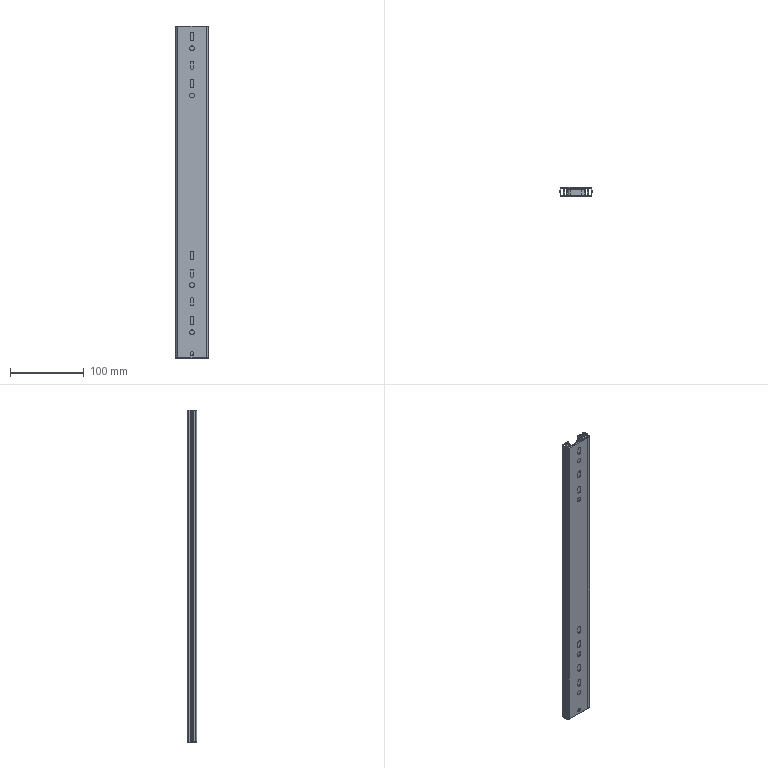Part | SolidWorks | features ICE 5, BossThin 2, LPattern 2, Chamfer 1, FlatPattern 1, SMBaseFlange 1, SheetMetal 1 | 2 solids | 222 faces | box 44.5 x 12.5 x 450 mm | volume 69033 mm3 | plane 125 | cylinder 86 | cone 11 | commonest cylinder face diameters 5 x29 2 x14 4 x14 6.5 x8 1.457 x6 3.457 x6